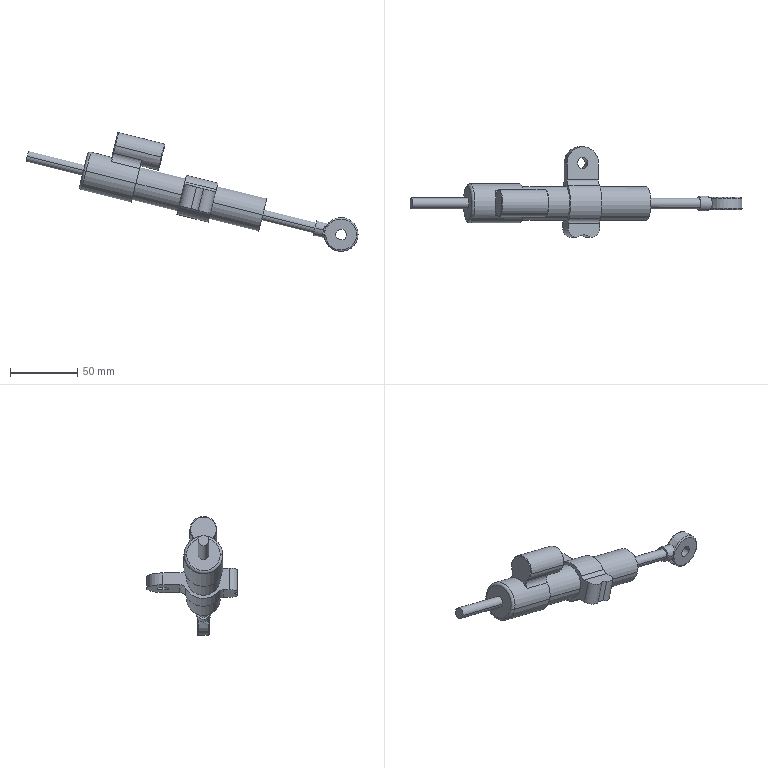Part | SolidWorks | features BaseBody 1 | 1 solid | 64 faces | box 246.341 x 67 x 88.196 mm | volume 108403 mm3 | cylinder 31 | plane 15 | torus 13 | spline 5 | commonest cylinder face diameters 8 x8 10 x7 25 x5 11 x2 12 x2 20 x2